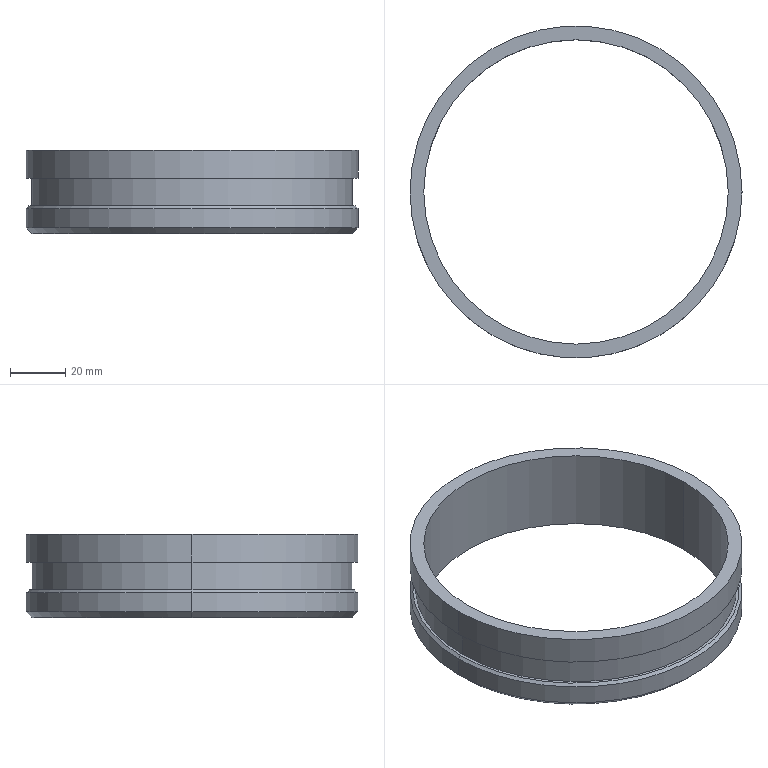Part | SolidWorks | features Chamfer 2, ICE 2, Extrusion 1 | 1 solid | 16 faces | box 120 x 120 x 30 mm | volume 45845 mm3 | cylinder 8 | cone 4 | plane 4 | commonest cylinder face diameters 120 x4 110 x2 116 x2
STEP:
#1=CARTESIAN_POINT('',(59.,0.,10.));
#2=VERTEX_POINT('',#1);
#3=CARTESIAN_POINT('',(-59.,0.,10.));
#4=VERTEX_POINT('',#3);
#5=CARTESIAN_POINT('',(0.,0.,10.));
#6=DIRECTION('',(0.,0.,1.));
#7=DIRECTION('',(1.,0.,0.));
#8=AXIS2_PLACEMENT_3D('',#5,#6,#7);
#9=CIRCLE('',#8,59.);
#10=EDGE_CURVE('',#2,#4,#9,.T.);
#11=ORIENTED_EDGE('',*,*,#10,.F.);
#12=CARTESIAN_POINT('',(60.,0.,9.));
#13=VERTEX_POINT('',#12);
#14=CARTESIAN_POINT('',(59.,0.,10.));
#15=DIRECTION('',(0.7071,0.,-0.7071));
#16=VECTOR('',#15,1000.);
#17=LINE('',#14,#16);
#18=EDGE_CURVE('',#2,#13,#17,.T.);
#19=ORIENTED_EDGE('',*,*,#18,.T.);
#20=CARTESIAN_POINT('',(-60.,0.,9.));
#21=VERTEX_POINT('',#20);
#22=CARTESIAN_POINT('',(0.,0.,9.));
#23=DIRECTION('',(0.,0.,-1.));
#24=DIRECTION('',(1.,0.,0.));
#25=AXIS2_PLACEMENT_3D('',#22,#23,#24);
#26=CIRCLE('',#25,60.);
#27=EDGE_CURVE('',#21,#13,#26,.T.);
#28=ORIENTED_EDGE('',*,*,#27,.F.);
#29=CARTESIAN_POINT('',(-59.,0.,10.));
#30=DIRECTION('',(-0.7071,0.,-0.7071));
#31=VECTOR('',#30,1000.);
#32=LINE('',#29,#31);
#33=EDGE_CURVE('',#4,#21,#32,.T.);
#34=ORIENTED_EDGE('',*,*,#33,.F.);
#35=EDGE_LOOP('',(#11,#19,#28,#34));
#36=FACE_OUTER_BOUND('',#35,.T.);
#37=CARTESIAN_POINT('',(0.,0.,10.));
#38=DIRECTION('',(0.,0.,-1.));
#39=DIRECTION('',(-1.,0.,0.));
#40=AXIS2_PLACEMENT_3D('',#37,#38,#39);
#41=CONICAL_SURFACE('',#40,59.,0.7854);
#42=ADVANCED_FACE('',(#36),#41,.T.);
#43=CARTESIAN_POINT('',(-58.,0.,0.));
#44=VERTEX_POINT('',#43);
#45=CARTESIAN_POINT('',(58.,0.,0.));
#46=VERTEX_POINT('',#45);
#47=CARTESIAN_POINT('',(0.,0.,0.));
#48=DIRECTION('',(0.,0.,-1.));
#49=DIRECTION('',(1.,0.,0.));
#50=AXIS2_PLACEMENT_3D('',#47,#48,#49);
#51=CIRCLE('',#50,58.);
#52=EDGE_CURVE('',#44,#46,#51,.T.);
#53=ORIENTED_EDGE('',*,*,#52,.F.);
#54=CARTESIAN_POINT('',(-60.,0.,2.));
#55=VERTEX_POINT('',#54);
#56=CARTESIAN_POINT('',(-60.,0.,2.));
#57=DIRECTION('',(-0.7071,0.,0.7071));
#58=VECTOR('',#57,1000.);
#59=LINE('',#56,#58);
#60=EDGE_CURVE('',#44,#55,#59,.T.);
#61=ORIENTED_EDGE('',*,*,#60,.T.);
#62=CARTESIAN_POINT('',(60.,0.,2.));
#63=VERTEX_POINT('',#62);
#64=CARTESIAN_POINT('',(0.,0.,2.));
#65=DIRECTION('',(0.,0.,1.));
#66=DIRECTION('',(1.,0.,0.));
#67=AXIS2_PLACEMENT_3D('',#64,#65,#66);
#68=CIRCLE('',#67,60.);
#69=EDGE_CURVE('',#63,#55,#68,.T.);
#70=ORIENTED_EDGE('',*,*,#69,.F.);
#71=CARTESIAN_POINT('',(60.,0.,2.));
#72=DIRECTION('',(0.7071,0.,0.7071));
#73=VECTOR('',#72,1000.);
#74=LINE('',#71,#73);
#75=EDGE_CURVE('',#46,#63,#74,.T.);
#76=ORIENTED_EDGE('',*,*,#75,.F.);
#77=EDGE_LOOP('',(#53,#61,#70,#76));
#78=FACE_OUTER_BOUND('',#77,.T.);
#79=CARTESIAN_POINT('',(0.,0.,2.));
#80=DIRECTION('',(0.,0.,1.));
#81=DIRECTION('',(1.,0.,0.));
#82=AXIS2_PLACEMENT_3D('',#79,#80,#81);
#83=CONICAL_SURFACE('',#82,60.,0.7854);
#84=ADVANCED_FACE('',(#78),#83,.T.);
#85=CARTESIAN_POINT('',(60.,0.,30.));
#86=VERTEX_POINT('',#85);
#87=CARTESIAN_POINT('',(-60.,0.,30.));
#88=VERTEX_POINT('',#87);
#89=CARTESIAN_POINT('',(0.,0.,30.));
#90=DIRECTION('',(0.,0.,1.));
#91=DIRECTION('',(1.,0.,0.));
#92=AXIS2_PLACEMENT_3D('',#89,#90,#91);
#93=CIRCLE('',#92,60.);
#94=EDGE_CURVE('',#86,#88,#93,.T.);
#95=ORIENTED_EDGE('',*,*,#94,.F.);
#96=CARTESIAN_POINT('',(60.,0.,20.));
#97=VERTEX_POINT('',#96);
#98=CARTESIAN_POINT('',(60.,0.,30.));
#99=DIRECTION('',(0.,0.,-1.));
#100=VECTOR('',#99,1000.);
#101=LINE('',#98,#100);
#102=EDGE_CURVE('',#86,#97,#101,.T.);
#103=ORIENTED_EDGE('',*,*,#102,.T.);
#104=CARTESIAN_POINT('',(-60.,0.,20.));
#105=VERTEX_POINT('',#104);
#106=CARTESIAN_POINT('',(0.,0.,20.));
#107=DIRECTION('',(0.,0.,1.));
#108=DIRECTION('',(1.,0.,0.));
#109=AXIS2_PLACEMENT_3D('',#106,#107,#108);
#110=CIRCLE('',#109,60.);
#111=EDGE_CURVE('',#97,#105,#110,.T.);
#112=ORIENTED_EDGE('',*,*,#111,.T.);
#113=CARTESIAN_POINT('',(-60.,0.,30.));
#114=DIRECTION('',(0.,0.,-1.));
#115=VECTOR('',#114,1000.);
#116=LINE('',#113,#115);
#117=EDGE_CURVE('',#88,#105,#116,.T.);
#118=ORIENTED_EDGE('',*,*,#117,.F.);
#119=EDGE_LOOP('',(#95,#103,#112,#118));
#120=FACE_OUTER_BOUND('',#119,.T.);
#121=CARTESIAN_POINT('',(0.,0.,30.));
#122=DIRECTION('',(0.,0.,-1.));
#123=DIRECTION('',(-1.,0.,0.));
#124=AXIS2_PLACEMENT_3D('',#121,#122,#123);
#125=CYLINDRICAL_SURFACE('',#124,60.);
#126=ADVANCED_FACE('',(#120),#125,.T.);
#127=CARTESIAN_POINT('',(58.,0.,10.));
#128=VERTEX_POINT('',#127);
#129=CARTESIAN_POINT('',(-58.,0.,10.));
#130=VERTEX_POINT('',#129);
#131=CARTESIAN_POINT('',(0.,0.,10.));
#132=DIRECTION('',(0.,0.,1.));
#133=DIRECTION('',(1.,0.,0.));
#134=AXIS2_PLACEMENT_3D('',#131,#132,#133);
#135=CIRCLE('',#134,58.);
#136=EDGE_CURVE('',#128,#130,#135,.T.);
#137=ORIENTED_EDGE('',*,*,#136,.T.);
#138=CARTESIAN_POINT('',(-58.,0.,20.));
#139=VERTEX_POINT('',#138);
#140=CARTESIAN_POINT('',(-58.,0.,10.));
#141=DIRECTION('',(0.,0.,1.));
#142=VECTOR('',#141,1000.);
#143=LINE('',#140,#142);
#144=EDGE_CURVE('',#130,#139,#143,.T.);
#145=ORIENTED_EDGE('',*,*,#144,.T.);
#146=CARTESIAN_POINT('',(58.,0.,20.));
#147=VERTEX_POINT('',#146);
#148=CARTESIAN_POINT('',(0.,0.,20.));
#149=DIRECTION('',(0.,0.,1.));
#150=DIRECTION('',(1.,0.,0.));
#151=AXIS2_PLACEMENT_3D('',#148,#149,#150);
#152=CIRCLE('',#151,58.);
#153=EDGE_CURVE('',#147,#139,#152,.T.);
#154=ORIENTED_EDGE('',*,*,#153,.F.);
#155=CARTESIAN_POINT('',(58.,0.,10.));
#156=DIRECTION('',(0.,0.,1.));
#157=VECTOR('',#156,1000.);
#158=LINE('',#155,#157);
#159=EDGE_CURVE('',#128,#147,#158,.T.);
#160=ORIENTED_EDGE('',*,*,#159,.F.);
#161=EDGE_LOOP('',(#137,#145,#154,#160));
#162=FACE_OUTER_BOUND('',#161,.T.);
#163=CARTESIAN_POINT('',(0.,0.,10.));
#164=DIRECTION('',(0.,0.,1.));
#165=DIRECTION('',(1.,0.,0.));
#166=AXIS2_PLACEMENT_3D('',#163,#164,#165);
#167=CYLINDRICAL_SURFACE('',#166,58.);
#168=ADVANCED_FACE('',(#162),#167,.T.);
#169=CARTESIAN_POINT('',(-55.,0.,30.));
#170=VERTEX_POINT('',#169);
#171=CARTESIAN_POINT('',(55.,0.,30.));
#172=VERTEX_POINT('',#171);
#173=CARTESIAN_POINT('',(0.,0.,30.));
#174=DIRECTION('',(0.,0.,1.));
#175=DIRECTION('',(1.,0.,0.));
#176=AXIS2_PLACEMENT_3D('',#173,#174,#175);
#177=CIRCLE('',#176,55.);
#178=EDGE_CURVE('',#170,#172,#177,.T.);
#179=ORIENTED_EDGE('',*,*,#178,.T.);
#180=CARTESIAN_POINT('',(55.,0.,0.));
#181=VERTEX_POINT('',#180);
#182=CARTESIAN_POINT('',(55.,0.,20.));
#183=DIRECTION('',(0.,0.,-1.));
#184=VECTOR('',#183,1000.);
#185=LINE('',#182,#184);
#186=EDGE_CURVE('',#172,#181,#185,.T.);
#187=ORIENTED_EDGE('',*,*,#186,.T.);
#188=CARTESIAN_POINT('',(-55.,0.,0.));
#189=VERTEX_POINT('',#188);
#190=CARTESIAN_POINT('',(0.,0.,0.));
#191=DIRECTION('',(0.,0.,1.));
#192=DIRECTION('',(1.,0.,0.));
#193=AXIS2_PLACEMENT_3D('',#190,#191,#192);
#194=CIRCLE('',#193,55.);
#195=EDGE_CURVE('',#189,#181,#194,.T.);
#196=ORIENTED_EDGE('',*,*,#195,.F.);
#197=CARTESIAN_POINT('',(-55.,0.,20.));
#198=DIRECTION('',(0.,0.,-1.));
#199=VECTOR('',#198,1000.);
#200=LINE('',#197,#199);
#201=EDGE_CURVE('',#170,#189,#200,.T.);
#202=ORIENTED_EDGE('',*,*,#201,.F.);
#203=EDGE_LOOP('',(#179,#187,#196,#202));
#204=FACE_OUTER_BOUND('',#203,.T.);
#205=CARTESIAN_POINT('',(0.,0.,20.));
#206=DIRECTION('',(0.,0.,-1.));
#207=DIRECTION('',(-1.,0.,0.));
#208=AXIS2_PLACEMENT_3D('',#205,#206,#207);
#209=CYLINDRICAL_SURFACE('',#208,55.);
#210=ADVANCED_FACE('',(#204),#209,.F.);
#211=ORIENTED_EDGE('',*,*,#27,.T.);
#212=CARTESIAN_POINT('',(60.,0.,20.));
#213=DIRECTION('',(0.,0.,-1.));
#214=VECTOR('',#213,1000.);
#215=LINE('',#212,#214);
#216=EDGE_CURVE('',#13,#63,#215,.T.);
#217=ORIENTED_EDGE('',*,*,#216,.T.);
#218=ORIENTED_EDGE('',*,*,#69,.T.);
#219=CARTESIAN_POINT('',(-60.,0.,20.));
#220=DIRECTION('',(0.,0.,-1.));
#221=VECTOR('',#220,1000.);
#222=LINE('',#219,#221);
#223=EDGE_CURVE('',#21,#55,#222,.T.);
#224=ORIENTED_EDGE('',*,*,#223,.F.);
#225=EDGE_LOOP('',(#211,#217,#218,#224));
#226=FACE_OUTER_BOUND('',#225,.T.);
#227=CARTESIAN_POINT('',(0.,0.,20.));
#228=DIRECTION('',(0.,0.,-1.));
#229=DIRECTION('',(-1.,0.,0.));
#230=AXIS2_PLACEMENT_3D('',#227,#228,#229);
#231=CYLINDRICAL_SURFACE('',#230,60.);
#232=ADVANCED_FACE('',(#226),#231,.T.);
#233=ORIENTED_EDGE('',*,*,#216,.F.);
#234=CARTESIAN_POINT('',(0.,0.,9.));
#235=DIRECTION('',(0.,0.,-1.));
#236=DIRECTION('',(1.,0.,0.));
#237=AXIS2_PLACEMENT_3D('',#234,#235,#236);
#238=CIRCLE('',#237,60.);
#239=EDGE_CURVE('',#13,#21,#238,.T.);
#240=ORIENTED_EDGE('',*,*,#239,.T.);
#241=ORIENTED_EDGE('',*,*,#223,.T.);
#242=CARTESIAN_POINT('',(0.,0.,2.));
#243=DIRECTION('',(0.,0.,1.));
#244=DIRECTION('',(1.,0.,0.));
#245=AXIS2_PLACEMENT_3D('',#242,#243,#244);
#246=CIRCLE('',#245,60.);
#247=EDGE_CURVE('',#55,#63,#246,.T.);
#248=ORIENTED_EDGE('',*,*,#247,.T.);
#249=EDGE_LOOP('',(#233,#240,#241,#248));
#250=FACE_OUTER_BOUND('',#249,.T.);
#251=CARTESIAN_POINT('',(0.,0.,20.));
#252=DIRECTION('',(0.,0.,-1.));
#253=DIRECTION('',(-1.,0.,0.));
#254=AXIS2_PLACEMENT_3D('',#251,#252,#253);
#255=CYLINDRICAL_SURFACE('',#254,60.);
#256=ADVANCED_FACE('',(#250),#255,.T.);
#257=CARTESIAN_POINT('',(0.,0.,0.));
#258=DIRECTION('',(0.,0.,-1.));
#259=DIRECTION('',(1.,0.,0.));
#260=AXIS2_PLACEMENT_3D('',#257,#258,#259);
#261=CIRCLE('',#260,58.);
#262=EDGE_CURVE('',#46,#44,#261,.T.);
#263=ORIENTED_EDGE('',*,*,#262,.T.);
#264=ORIENTED_EDGE('',*,*,#52,.T.);
#265=EDGE_LOOP('',(#263,#264));
#266=FACE_OUTER_BOUND('',#265,.T.);
#267=ORIENTED_EDGE('',*,*,#195,.T.);
#268=CARTESIAN_POINT('',(0.,0.,0.));
#269=DIRECTION('',(0.,0.,1.));
#270=DIRECTION('',(1.,0.,0.));
#271=AXIS2_PLACEMENT_3D('',#268,#269,#270);
#272=CIRCLE('',#271,55.);
#273=EDGE_CURVE('',#181,#189,#272,.T.);
#274=ORIENTED_EDGE('',*,*,#273,.T.);
#275=EDGE_LOOP('',(#267,#274));
#276=FACE_BOUND('',#275,.T.);
#277=CARTESIAN_POINT('',(0.,0.,0.));
#278=DIRECTION('',(0.,0.,1.));
#279=DIRECTION('',(1.,0.,0.));
#280=AXIS2_PLACEMENT_3D('',#277,#278,#279);
#281=PLANE('',#280);
#282=ADVANCED_FACE('',(#266,#276),#281,.F.);
#283=ORIENTED_EDGE('',*,*,#186,.F.);
#284=CARTESIAN_POINT('',(0.,0.,30.));
#285=DIRECTION('',(0.,0.,1.));
#286=DIRECTION('',(1.,0.,0.));
#287=AXIS2_PLACEMENT_3D('',#284,#285,#286);
#288=CIRCLE('',#287,55.);
#289=EDGE_CURVE('',#172,#170,#288,.T.);
#290=ORIENTED_EDGE('',*,*,#289,.T.);
#291=ORIENTED_EDGE('',*,*,#201,.T.);
#292=ORIENTED_EDGE('',*,*,#273,.F.);
#293=EDGE_LOOP('',(#283,#290,#291,#292));
#294=FACE_OUTER_BOUND('',#293,.T.);
#295=CARTESIAN_POINT('',(0.,0.,20.));
#296=DIRECTION('',(0.,0.,-1.));
#297=DIRECTION('',(-1.,0.,0.));
#298=AXIS2_PLACEMENT_3D('',#295,#296,#297);
#299=CYLINDRICAL_SURFACE('',#298,55.);
#300=ADVANCED_FACE('',(#294),#299,.F.);
#301=CARTESIAN_POINT('',(0.,0.,10.));
#302=DIRECTION('',(0.,0.,1.));
#303=DIRECTION('',(1.,0.,0.));
#304=AXIS2_PLACEMENT_3D('',#301,#302,#303);
#305=CIRCLE('',#304,59.);
#306=EDGE_CURVE('',#4,#2,#305,.T.);
#307=ORIENTED_EDGE('',*,*,#306,.T.);
#308=ORIENTED_EDGE('',*,*,#10,.T.);
#309=EDGE_LOOP('',(#307,#308));
#310=FACE_OUTER_BOUND('',#309,.T.);
#311=ORIENTED_EDGE('',*,*,#136,.F.);
#312=CARTESIAN_POINT('',(0.,0.,10.));
#313=DIRECTION('',(0.,0.,1.));
#314=DIRECTION('',(1.,0.,0.));
#315=AXIS2_PLACEMENT_3D('',#312,#313,#314);
#316=CIRCLE('',#315,58.);
#317=EDGE_CURVE('',#130,#128,#316,.T.);
#318=ORIENTED_EDGE('',*,*,#317,.F.);
#319=EDGE_LOOP('',(#311,#318));
#320=FACE_BOUND('',#319,.T.);
#321=CARTESIAN_POINT('',(0.,0.,10.));
#322=DIRECTION('',(0.,0.,1.));
#323=DIRECTION('',(1.,0.,0.));
#324=AXIS2_PLACEMENT_3D('',#321,#322,#323);
#325=PLANE('',#324);
#326=ADVANCED_FACE('',(#310,#320),#325,.T.);
#327=ORIENTED_EDGE('',*,*,#144,.F.);
#328=ORIENTED_EDGE('',*,*,#317,.T.);
#329=ORIENTED_EDGE('',*,*,#159,.T.);
#330=CARTESIAN_POINT('',(0.,0.,20.));
#331=DIRECTION('',(0.,0.,1.));
#332=DIRECTION('',(1.,0.,0.));
#333=AXIS2_PLACEMENT_3D('',#330,#331,#332);
#334=CIRCLE('',#333,58.);
#335=EDGE_CURVE('',#139,#147,#334,.T.);
#336=ORIENTED_EDGE('',*,*,#335,.F.);
#337=EDGE_LOOP('',(#327,#328,#329,#336));
#338=FACE_OUTER_BOUND('',#337,.T.);
#339=CARTESIAN_POINT('',(0.,0.,10.));
#340=DIRECTION('',(0.,0.,1.));
#341=DIRECTION('',(1.,0.,0.));
#342=AXIS2_PLACEMENT_3D('',#339,#340,#341);
#343=CYLINDRICAL_SURFACE('',#342,58.);
#344=ADVANCED_FACE('',(#338),#343,.T.);
#345=CARTESIAN_POINT('',(0.,0.,30.));
#346=DIRECTION('',(0.,0.,1.));
#347=DIRECTION('',(1.,0.,0.));
#348=AXIS2_PLACEMENT_3D('',#345,#346,#347);
#349=CIRCLE('',#348,60.);
#350=EDGE_CURVE('',#88,#86,#349,.T.);
#351=ORIENTED_EDGE('',*,*,#350,.T.);
#352=ORIENTED_EDGE('',*,*,#94,.T.);
#353=EDGE_LOOP('',(#351,#352));
#354=FACE_OUTER_BOUND('',#353,.T.);
#355=ORIENTED_EDGE('',*,*,#178,.F.);
#356=ORIENTED_EDGE('',*,*,#289,.F.);
#357=EDGE_LOOP('',(#355,#356));
#358=FACE_BOUND('',#357,.T.);
#359=CARTESIAN_POINT('',(0.,0.,30.));
#360=DIRECTION('',(0.,0.,1.));
#361=DIRECTION('',(1.,0.,0.));
#362=AXIS2_PLACEMENT_3D('',#359,#360,#361);
#363=PLANE('',#362);
#364=ADVANCED_FACE('',(#354,#358),#363,.T.);
#365=ORIENTED_EDGE('',*,*,#153,.T.);
#366=ORIENTED_EDGE('',*,*,#335,.T.);
#367=EDGE_LOOP('',(#365,#366));
#368=FACE_BOUND('',#367,.T.);
#369=CARTESIAN_POINT('',(0.,0.,20.));
#370=DIRECTION('',(0.,0.,1.));
#371=DIRECTION('',(1.,0.,0.));
#372=AXIS2_PLACEMENT_3D('',#369,#370,#371);
#373=CIRCLE('',#372,60.);
#374=EDGE_CURVE('',#105,#97,#373,.T.);
#375=ORIENTED_EDGE('',*,*,#374,.F.);
#376=ORIENTED_EDGE('',*,*,#111,.F.);
#377=EDGE_LOOP('',(#375,#376));
#378=FACE_OUTER_BOUND('',#377,.T.);
#379=CARTESIAN_POINT('',(0.,0.,20.));
#380=DIRECTION('',(0.,0.,1.));
#381=DIRECTION('',(1.,0.,0.));
#382=AXIS2_PLACEMENT_3D('',#379,#380,#381);
#383=PLANE('',#382);
#384=ADVANCED_FACE('',(#368,#378),#383,.F.);
#385=ORIENTED_EDGE('',*,*,#102,.F.);
#386=ORIENTED_EDGE('',*,*,#350,.F.);
#387=ORIENTED_EDGE('',*,*,#117,.T.);
#388=ORIENTED_EDGE('',*,*,#374,.T.);
#389=EDGE_LOOP('',(#385,#386,#387,#388));
#390=FACE_OUTER_BOUND('',#389,.T.);
#391=CARTESIAN_POINT('',(0.,0.,30.));
#392=DIRECTION('',(0.,0.,-1.));
#393=DIRECTION('',(-1.,0.,0.));
#394=AXIS2_PLACEMENT_3D('',#391,#392,#393);
#395=CYLINDRICAL_SURFACE('',#394,60.);
#396=ADVANCED_FACE('',(#390),#395,.T.);
#397=ORIENTED_EDGE('',*,*,#60,.F.);
#398=ORIENTED_EDGE('',*,*,#262,.F.);
#399=ORIENTED_EDGE('',*,*,#75,.T.);
#400=ORIENTED_EDGE('',*,*,#247,.F.);
#401=EDGE_LOOP('',(#397,#398,#399,#400));
#402=FACE_OUTER_BOUND('',#401,.T.);
#403=CARTESIAN_POINT('',(0.,0.,2.));
#404=DIRECTION('',(0.,0.,1.));
#405=DIRECTION('',(1.,0.,0.));
#406=AXIS2_PLACEMENT_3D('',#403,#404,#405);
#407=CONICAL_SURFACE('',#406,60.,0.7854);
#408=ADVANCED_FACE('',(#402),#407,.T.);
#409=ORIENTED_EDGE('',*,*,#18,.F.);
#410=ORIENTED_EDGE('',*,*,#306,.F.);
#411=ORIENTED_EDGE('',*,*,#33,.T.);
#412=ORIENTED_EDGE('',*,*,#239,.F.);
#413=EDGE_LOOP('',(#409,#410,#411,#412));
#414=FACE_OUTER_BOUND('',#413,.T.);
#415=CARTESIAN_POINT('',(0.,0.,10.));
#416=DIRECTION('',(0.,0.,-1.));
#417=DIRECTION('',(-1.,0.,0.));
#418=AXIS2_PLACEMENT_3D('',#415,#416,#417);
#419=CONICAL_SURFACE('',#418,59.,0.7854);
#420=ADVANCED_FACE('',(#414),#419,.T.);
#421=CLOSED_SHELL('',(#42,#84,#126,#168,#210,#232,#256,#282,#300,#326,#344,#364,#384,#396,#408,#420));
#422=MANIFOLD_SOLID_BREP('',#421);
#423=CARTESIAN_POINT('',(0.,0.,0.));
#424=DIRECTION('',(0.,0.,1.));
#425=DIRECTION('',(1.,0.,0.));
#426=AXIS2_PLACEMENT_3D('',#423,#424,#425);
#427=(LENGTH_UNIT()NAMED_UNIT(*)SI_UNIT(.MILLI.,.METRE.));
#428=UNCERTAINTY_MEASURE_WITH_UNIT(LENGTH_MEASURE(0.00001),#427,'','');
#429=(NAMED_UNIT(*)PLANE_ANGLE_UNIT()SI_UNIT($,.RADIAN.));
#430=(NAMED_UNIT(*)SI_UNIT($,.STERADIAN.)SOLID_ANGLE_UNIT());
#431=(GEOMETRIC_REPRESENTATION_CONTEXT(3)GLOBAL_UNCERTAINTY_ASSIGNED_CONTEXT((#428))GLOBAL_UNIT_ASSIGNED_CONTEXT((#427,#429,#430))REPRESENTATION_CONTEXT('',''));
#432=ADVANCED_BREP_SHAPE_REPRESENTATION('',(#422,#426),#431);